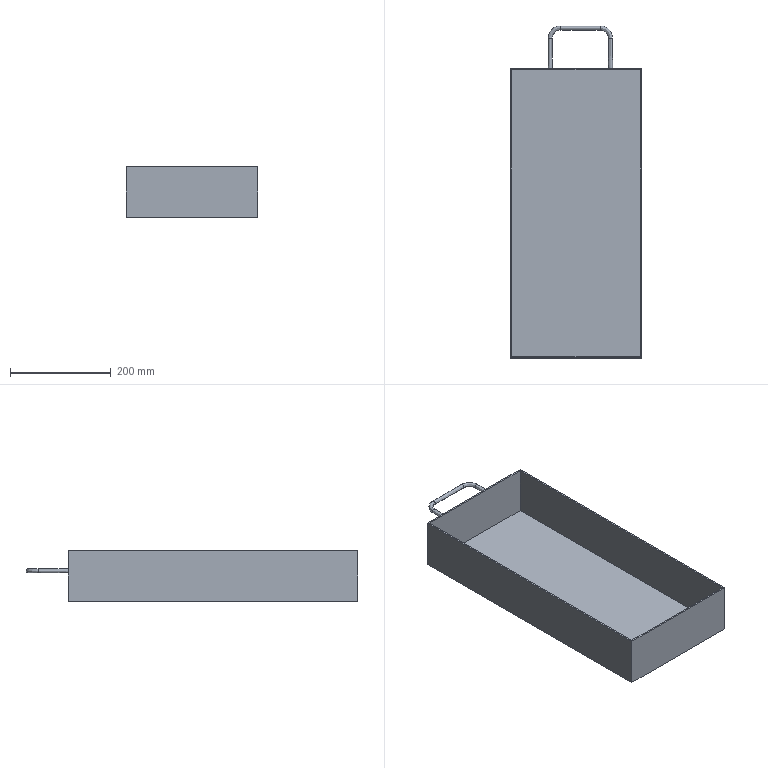Part | NX | features solid 2 | 1 solid | 16 faces | box 261 x 659 x 100 mm | volume 946502 mm3 | plane 11 | spline 5